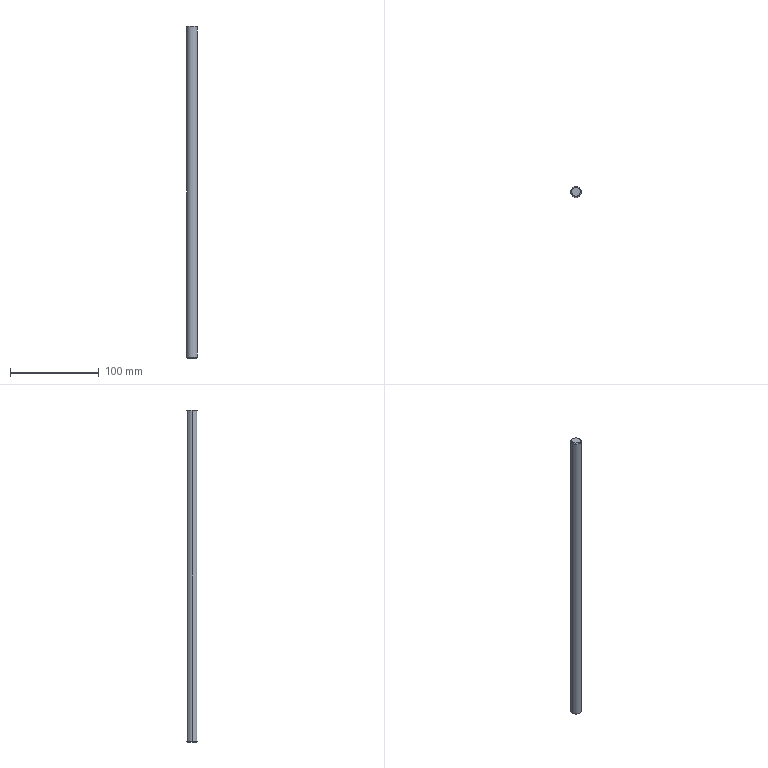Part | SolidWorks | features BaseBody 1 | 1 solid | 20 faces | box 12 x 12 x 374 mm | volume 42082 mm3 | cylinder 8 | plane 8 | cone 4 | commonest cylinder face diameters 3 x6 12 x2
STEP:
#1=CARTESIAN_POINT('',(4.2,0.,-179.));
#2=VERTEX_POINT('',#1);
#3=CARTESIAN_POINT('',(4.2,1.5,-177.5));
#4=VERTEX_POINT('',#3);
#5=CARTESIAN_POINT('',(4.2,0.,-177.5));
#6=DIRECTION('',(1.,0.,0.));
#7=DIRECTION('',(0.,0.,-1.));
#8=AXIS2_PLACEMENT_3D('',#5,#6,#7);
#9=CIRCLE('',#8,1.5);
#10=EDGE_CURVE('',#2,#4,#9,.T.);
#11=ORIENTED_EDGE('',*,*,#10,.F.);
#12=CARTESIAN_POINT('',(6.,0.,-179.));
#13=VERTEX_POINT('',#12);
#14=CARTESIAN_POINT('',(4.2,0.,-179.));
#15=DIRECTION('',(1.,0.,0.));
#16=VECTOR('',#15,1000.);
#17=LINE('',#14,#16);
#18=EDGE_CURVE('',#2,#13,#17,.T.);
#19=ORIENTED_EDGE('',*,*,#18,.T.);
#20=CARTESIAN_POINT('',(5.809,1.5,-177.5));
#21=VERTEX_POINT('',#20);
#22=CARTESIAN_POINT('',(5.809,1.5,-177.5));
#23=CARTESIAN_POINT('',(5.809,1.5,-177.6));
#24=CARTESIAN_POINT('',(5.812,1.49,-177.697));
#25=CARTESIAN_POINT('',(5.822,1.452,-177.89));
#26=CARTESIAN_POINT('',(5.829,1.423,-177.985));
#27=CARTESIAN_POINT('',(5.847,1.347,-178.167));
#28=CARTESIAN_POINT('',(5.857,1.301,-178.253));
#29=CARTESIAN_POINT('',(5.881,1.192,-178.415));
#30=CARTESIAN_POINT('',(5.893,1.129,-178.492));
#31=CARTESIAN_POINT('',(5.93,0.9223,-178.699));
#32=CARTESIAN_POINT('',(5.955,0.7555,-178.81));
#33=CARTESIAN_POINT('',(5.99,0.3946,-178.96));
#34=CARTESIAN_POINT('',(6.,0.1966,-179.));
#35=CARTESIAN_POINT('',(6.,0.,-179.));
#36=B_SPLINE_CURVE_WITH_KNOTS('',3,(#22,#23,#24,#25,#26,#27,#28,#29,#30,#31,#32,#33,#34,#35),.UNSPECIFIED.,.F.,.F.,(4,2,2,2,2,2,4),(0.,0.0002944,0.0005887,0.0008831,0.001177,0.001766,0.002355),.UNSPECIFIED.);
#37=EDGE_CURVE('',#21,#13,#36,.T.);
#38=ORIENTED_EDGE('',*,*,#37,.F.);
#39=CARTESIAN_POINT('',(4.2,1.5,-177.5));
#40=DIRECTION('',(1.,0.,0.));
#41=VECTOR('',#40,1000.);
#42=LINE('',#39,#41);
#43=EDGE_CURVE('',#4,#21,#42,.T.);
#44=ORIENTED_EDGE('',*,*,#43,.F.);
#45=EDGE_LOOP('',(#11,#19,#38,#44));
#46=FACE_OUTER_BOUND('',#45,.T.);
#47=CARTESIAN_POINT('',(4.2,0.,-177.5));
#48=DIRECTION('',(1.,0.,0.));
#49=DIRECTION('',(0.,0.,-1.));
#50=AXIS2_PLACEMENT_3D('',#47,#48,#49);
#51=CYLINDRICAL_SURFACE('',#50,1.5);
#52=ADVANCED_FACE('',(#46),#51,.F.);
#53=CARTESIAN_POINT('',(4.2,0.,161.));
#54=VERTEX_POINT('',#53);
#55=CARTESIAN_POINT('',(4.2,1.5,162.5));
#56=VERTEX_POINT('',#55);
#57=CARTESIAN_POINT('',(4.2,0.,162.5));
#58=DIRECTION('',(1.,0.,0.));
#59=DIRECTION('',(0.,0.,1.));
#60=AXIS2_PLACEMENT_3D('',#57,#58,#59);
#61=CIRCLE('',#60,1.5);
#62=EDGE_CURVE('',#54,#56,#61,.T.);
#63=ORIENTED_EDGE('',*,*,#62,.F.);
#64=CARTESIAN_POINT('',(6.,0.,161.));
#65=VERTEX_POINT('',#64);
#66=CARTESIAN_POINT('',(4.2,0.,161.));
#67=DIRECTION('',(1.,0.,0.));
#68=VECTOR('',#67,1000.);
#69=LINE('',#66,#68);
#70=EDGE_CURVE('',#54,#65,#69,.T.);
#71=ORIENTED_EDGE('',*,*,#70,.T.);
#72=CARTESIAN_POINT('',(5.809,1.5,162.5));
#73=VERTEX_POINT('',#72);
#74=CARTESIAN_POINT('',(5.809,1.5,162.5));
#75=CARTESIAN_POINT('',(5.809,1.5,162.4));
#76=CARTESIAN_POINT('',(5.812,1.49,162.303));
#77=CARTESIAN_POINT('',(5.822,1.452,162.11));
#78=CARTESIAN_POINT('',(5.829,1.423,162.015));
#79=CARTESIAN_POINT('',(5.847,1.347,161.833));
#80=CARTESIAN_POINT('',(5.857,1.301,161.747));
#81=CARTESIAN_POINT('',(5.881,1.192,161.585));
#82=CARTESIAN_POINT('',(5.893,1.129,161.508));
#83=CARTESIAN_POINT('',(5.93,0.9223,161.301));
#84=CARTESIAN_POINT('',(5.955,0.7555,161.19));
#85=CARTESIAN_POINT('',(5.99,0.3946,161.04));
#86=CARTESIAN_POINT('',(6.,0.1966,161.));
#87=CARTESIAN_POINT('',(6.,0.,161.));
#88=B_SPLINE_CURVE_WITH_KNOTS('',3,(#74,#75,#76,#77,#78,#79,#80,#81,#82,#83,#84,#85,#86,#87),.UNSPECIFIED.,.F.,.F.,(4,2,2,2,2,2,4),(0.,0.0002944,0.0005887,0.0008831,0.001177,0.001766,0.002355),.UNSPECIFIED.);
#89=EDGE_CURVE('',#73,#65,#88,.T.);
#90=ORIENTED_EDGE('',*,*,#89,.F.);
#91=CARTESIAN_POINT('',(4.2,1.5,162.5));
#92=DIRECTION('',(1.,0.,0.));
#93=VECTOR('',#92,1000.);
#94=LINE('',#91,#93);
#95=EDGE_CURVE('',#56,#73,#94,.T.);
#96=ORIENTED_EDGE('',*,*,#95,.F.);
#97=EDGE_LOOP('',(#63,#71,#90,#96));
#98=FACE_OUTER_BOUND('',#97,.T.);
#99=CARTESIAN_POINT('',(4.2,0.,162.5));
#100=DIRECTION('',(1.,0.,0.));
#101=DIRECTION('',(0.,0.,-1.));
#102=AXIS2_PLACEMENT_3D('',#99,#100,#101);
#103=CYLINDRICAL_SURFACE('',#102,1.5);
#104=ADVANCED_FACE('',(#98),#103,.F.);
#105=CARTESIAN_POINT('',(-5.,0.,-187.));
#106=VERTEX_POINT('',#105);
#107=CARTESIAN_POINT('',(5.,0.,-187.));
#108=VERTEX_POINT('',#107);
#109=CARTESIAN_POINT('',(0.,0.,-187.));
#110=DIRECTION('',(0.,0.,-1.));
#111=DIRECTION('',(1.,0.,0.));
#112=AXIS2_PLACEMENT_3D('',#109,#110,#111);
#113=CIRCLE('',#112,5.);
#114=EDGE_CURVE('',#106,#108,#113,.T.);
#115=ORIENTED_EDGE('',*,*,#114,.F.);
#116=CARTESIAN_POINT('',(-6.,0.,-186.));
#117=VERTEX_POINT('',#116);
#118=CARTESIAN_POINT('',(-6.,0.,-186.));
#119=DIRECTION('',(-0.7071,0.,0.7071));
#120=VECTOR('',#119,1000.);
#121=LINE('',#118,#120);
#122=EDGE_CURVE('',#106,#117,#121,.T.);
#123=ORIENTED_EDGE('',*,*,#122,.T.);
#124=CARTESIAN_POINT('',(6.,0.,-186.));
#125=VERTEX_POINT('',#124);
#126=CARTESIAN_POINT('',(0.,0.,-186.));
#127=DIRECTION('',(0.,0.,1.));
#128=DIRECTION('',(1.,0.,0.));
#129=AXIS2_PLACEMENT_3D('',#126,#127,#128);
#130=CIRCLE('',#129,6.);
#131=EDGE_CURVE('',#125,#117,#130,.T.);
#132=ORIENTED_EDGE('',*,*,#131,.F.);
#133=CARTESIAN_POINT('',(6.,0.,-186.));
#134=DIRECTION('',(0.7071,0.,0.7071));
#135=VECTOR('',#134,1000.);
#136=LINE('',#133,#135);
#137=EDGE_CURVE('',#108,#125,#136,.T.);
#138=ORIENTED_EDGE('',*,*,#137,.F.);
#139=EDGE_LOOP('',(#115,#123,#132,#138));
#140=FACE_OUTER_BOUND('',#139,.T.);
#141=CARTESIAN_POINT('',(0.,0.,-186.));
#142=DIRECTION('',(0.,0.,1.));
#143=DIRECTION('',(1.,0.,0.));
#144=AXIS2_PLACEMENT_3D('',#141,#142,#143);
#145=CONICAL_SURFACE('',#144,6.,0.7854);
#146=ADVANCED_FACE('',(#140),#145,.T.);
#147=CARTESIAN_POINT('',(5.,0.,187.));
#148=VERTEX_POINT('',#147);
#149=CARTESIAN_POINT('',(-5.,0.,187.));
#150=VERTEX_POINT('',#149);
#151=CARTESIAN_POINT('',(0.,0.,187.));
#152=DIRECTION('',(0.,0.,1.));
#153=DIRECTION('',(1.,0.,0.));
#154=AXIS2_PLACEMENT_3D('',#151,#152,#153);
#155=CIRCLE('',#154,5.);
#156=EDGE_CURVE('',#148,#150,#155,.T.);
#157=ORIENTED_EDGE('',*,*,#156,.F.);
#158=CARTESIAN_POINT('',(6.,0.,186.));
#159=VERTEX_POINT('',#158);
#160=CARTESIAN_POINT('',(5.,0.,187.));
#161=DIRECTION('',(0.7071,0.,-0.7071));
#162=VECTOR('',#161,1000.);
#163=LINE('',#160,#162);
#164=EDGE_CURVE('',#148,#159,#163,.T.);
#165=ORIENTED_EDGE('',*,*,#164,.T.);
#166=CARTESIAN_POINT('',(-6.,0.,186.));
#167=VERTEX_POINT('',#166);
#168=CARTESIAN_POINT('',(0.,0.,186.));
#169=DIRECTION('',(0.,0.,-1.));
#170=DIRECTION('',(1.,0.,0.));
#171=AXIS2_PLACEMENT_3D('',#168,#169,#170);
#172=CIRCLE('',#171,6.);
#173=EDGE_CURVE('',#167,#159,#172,.T.);
#174=ORIENTED_EDGE('',*,*,#173,.F.);
#175=CARTESIAN_POINT('',(-5.,0.,187.));
#176=DIRECTION('',(-0.7071,0.,-0.7071));
#177=VECTOR('',#176,1000.);
#178=LINE('',#175,#177);
#179=EDGE_CURVE('',#150,#167,#178,.T.);
#180=ORIENTED_EDGE('',*,*,#179,.F.);
#181=EDGE_LOOP('',(#157,#165,#174,#180));
#182=FACE_OUTER_BOUND('',#181,.T.);
#183=CARTESIAN_POINT('',(0.,0.,187.));
#184=DIRECTION('',(0.,0.,-1.));
#185=DIRECTION('',(-1.,0.,0.));
#186=AXIS2_PLACEMENT_3D('',#183,#184,#185);
#187=CONICAL_SURFACE('',#186,5.,0.7854);
#188=ADVANCED_FACE('',(#182),#187,.T.);
#189=ORIENTED_EDGE('',*,*,#173,.T.);
#190=CARTESIAN_POINT('',(6.,0.,179.));
#191=VERTEX_POINT('',#190);
#192=CARTESIAN_POINT('',(6.,0.,187.));
#193=DIRECTION('',(0.,0.,-1.));
#194=VECTOR('',#193,1000.);
#195=LINE('',#192,#194);
#196=EDGE_CURVE('',#159,#191,#195,.T.);
#197=ORIENTED_EDGE('',*,*,#196,.T.);
#198=CARTESIAN_POINT('',(5.809,1.5,177.5));
#199=VERTEX_POINT('',#198);
#200=CARTESIAN_POINT('',(6.,0.,179.));
#201=CARTESIAN_POINT('',(6.,0.1962,179.));
#202=CARTESIAN_POINT('',(5.99,0.3944,178.96));
#203=CARTESIAN_POINT('',(5.964,0.6654,178.848));
#204=CARTESIAN_POINT('',(5.953,0.7532,178.801));
#205=CARTESIAN_POINT('',(5.93,0.916,178.692));
#206=CARTESIAN_POINT('',(5.918,0.9912,178.63));
#207=CARTESIAN_POINT('',(5.893,1.13,178.492));
#208=CARTESIAN_POINT('',(5.881,1.193,178.415));
#209=CARTESIAN_POINT('',(5.858,1.301,178.253));
#210=CARTESIAN_POINT('',(5.847,1.347,178.167));
#211=CARTESIAN_POINT('',(5.82,1.461,177.893));
#212=CARTESIAN_POINT('',(5.809,1.5,177.698));
#213=CARTESIAN_POINT('',(5.809,1.5,177.5));
#214=B_SPLINE_CURVE_WITH_KNOTS('',3,(#200,#201,#202,#203,#204,#205,#206,#207,#208,#209,#210,#211,#212,#213),.UNSPECIFIED.,.F.,.F.,(4,2,2,2,2,2,4),(0.004708,0.005297,0.005591,0.005885,0.00618,0.006474,0.007062),.UNSPECIFIED.);
#215=EDGE_CURVE('',#191,#199,#214,.T.);
#216=ORIENTED_EDGE('',*,*,#215,.T.);
#217=CARTESIAN_POINT('',(5.809,1.5,187.));
#218=DIRECTION('',(0.,0.,-1.));
#219=VECTOR('',#218,1000.);
#220=LINE('',#217,#219);
#221=EDGE_CURVE('',#199,#73,#220,.T.);
#222=ORIENTED_EDGE('',*,*,#221,.T.);
#223=ORIENTED_EDGE('',*,*,#89,.T.);
#224=CARTESIAN_POINT('',(6.,0.,-161.));
#225=VERTEX_POINT('',#224);
#226=CARTESIAN_POINT('',(6.,0.,187.));
#227=DIRECTION('',(0.,0.,-1.));
#228=VECTOR('',#227,1000.);
#229=LINE('',#226,#228);
#230=EDGE_CURVE('',#65,#225,#229,.T.);
#231=ORIENTED_EDGE('',*,*,#230,.T.);
#232=CARTESIAN_POINT('',(5.809,1.5,-162.5));
#233=VERTEX_POINT('',#232);
#234=CARTESIAN_POINT('',(6.,0.,-161.));
#235=CARTESIAN_POINT('',(6.,0.1962,-161.));
#236=CARTESIAN_POINT('',(5.99,0.3944,-161.04));
#237=CARTESIAN_POINT('',(5.964,0.6654,-161.152));
#238=CARTESIAN_POINT('',(5.953,0.7532,-161.199));
#239=CARTESIAN_POINT('',(5.93,0.916,-161.308));
#240=CARTESIAN_POINT('',(5.918,0.9912,-161.37));
#241=CARTESIAN_POINT('',(5.893,1.13,-161.508));
#242=CARTESIAN_POINT('',(5.881,1.193,-161.585));
#243=CARTESIAN_POINT('',(5.858,1.301,-161.747));
#244=CARTESIAN_POINT('',(5.847,1.347,-161.833));
#245=CARTESIAN_POINT('',(5.82,1.461,-162.107));
#246=CARTESIAN_POINT('',(5.809,1.5,-162.302));
#247=CARTESIAN_POINT('',(5.809,1.5,-162.5));
#248=B_SPLINE_CURVE_WITH_KNOTS('',3,(#234,#235,#236,#237,#238,#239,#240,#241,#242,#243,#244,#245,#246,#247),.UNSPECIFIED.,.F.,.F.,(4,2,2,2,2,2,4),(0.004708,0.005297,0.005591,0.005885,0.00618,0.006474,0.007062),.UNSPECIFIED.);
#249=EDGE_CURVE('',#225,#233,#248,.T.);
#250=ORIENTED_EDGE('',*,*,#249,.T.);
#251=CARTESIAN_POINT('',(5.809,1.5,187.));
#252=DIRECTION('',(0.,0.,-1.));
#253=VECTOR('',#252,1000.);
#254=LINE('',#251,#253);
#255=EDGE_CURVE('',#233,#21,#254,.T.);
#256=ORIENTED_EDGE('',*,*,#255,.T.);
#257=ORIENTED_EDGE('',*,*,#37,.T.);
#258=CARTESIAN_POINT('',(6.,0.,187.));
#259=DIRECTION('',(0.,0.,-1.));
#260=VECTOR('',#259,1000.);
#261=LINE('',#258,#260);
#262=EDGE_CURVE('',#13,#125,#261,.T.);
#263=ORIENTED_EDGE('',*,*,#262,.T.);
#264=ORIENTED_EDGE('',*,*,#131,.T.);
#265=CARTESIAN_POINT('',(-6.,0.,187.));
#266=DIRECTION('',(0.,0.,-1.));
#267=VECTOR('',#266,1000.);
#268=LINE('',#265,#267);
#269=EDGE_CURVE('',#167,#117,#268,.T.);
#270=ORIENTED_EDGE('',*,*,#269,.F.);
#271=EDGE_LOOP('',(#189,#197,#216,#222,#223,#231,#250,#256,#257,#263,#264,#270));
#272=FACE_OUTER_BOUND('',#271,.T.);
#273=CARTESIAN_POINT('',(0.,0.,187.));
#274=DIRECTION('',(0.,0.,-1.));
#275=DIRECTION('',(-1.,0.,0.));
#276=AXIS2_PLACEMENT_3D('',#273,#274,#275);
#277=CYLINDRICAL_SURFACE('',#276,6.);
#278=ADVANCED_FACE('',(#272),#277,.T.);
#279=ORIENTED_EDGE('',*,*,#196,.F.);
#280=CARTESIAN_POINT('',(0.,0.,186.));
#281=DIRECTION('',(0.,0.,-1.));
#282=DIRECTION('',(1.,0.,0.));
#283=AXIS2_PLACEMENT_3D('',#280,#281,#282);
#284=CIRCLE('',#283,6.);
#285=EDGE_CURVE('',#159,#167,#284,.T.);
#286=ORIENTED_EDGE('',*,*,#285,.T.);
#287=ORIENTED_EDGE('',*,*,#269,.T.);
#288=CARTESIAN_POINT('',(0.,0.,-186.));
#289=DIRECTION('',(0.,0.,1.));
#290=DIRECTION('',(1.,0.,0.));
#291=AXIS2_PLACEMENT_3D('',#288,#289,#290);
#292=CIRCLE('',#291,6.);
#293=EDGE_CURVE('',#117,#125,#292,.T.);
#294=ORIENTED_EDGE('',*,*,#293,.T.);
#295=ORIENTED_EDGE('',*,*,#262,.F.);
#296=CARTESIAN_POINT('',(5.809,-1.5,-177.5));
#297=VERTEX_POINT('',#296);
#298=CARTESIAN_POINT('',(6.,0.,-179.));
#299=CARTESIAN_POINT('',(6.,-0.0982,-179.));
#300=CARTESIAN_POINT('',(5.998,-0.198,-178.99));
#301=CARTESIAN_POINT('',(5.988,-0.3905,-178.952));
#302=CARTESIAN_POINT('',(5.981,-0.4841,-178.923));
#303=CARTESIAN_POINT('',(5.955,-0.7571,-178.81));
#304=CARTESIAN_POINT('',(5.93,-0.9218,-178.699));
#305=CARTESIAN_POINT('',(5.893,-1.13,-178.491));
#306=CARTESIAN_POINT('',(5.881,-1.192,-178.416));
#307=CARTESIAN_POINT('',(5.858,-1.3,-178.254));
#308=CARTESIAN_POINT('',(5.847,-1.347,-178.166));
#309=CARTESIAN_POINT('',(5.82,-1.46,-177.895));
#310=CARTESIAN_POINT('',(5.809,-1.5,-177.699));
#311=CARTESIAN_POINT('',(5.809,-1.5,-177.5));
#312=B_SPLINE_CURVE_WITH_KNOTS('',3,(#298,#299,#300,#301,#302,#303,#304,#305,#306,#307,#308,#309,#310,#311),.UNSPECIFIED.,.F.,.F.,(4,2,2,2,2,2,4),(0.002355,0.002649,0.002943,0.003531,0.003825,0.004119,0.004707),.UNSPECIFIED.);
#313=EDGE_CURVE('',#13,#297,#312,.T.);
#314=ORIENTED_EDGE('',*,*,#313,.T.);
#315=CARTESIAN_POINT('',(5.809,-1.5,-162.5));
#316=VERTEX_POINT('',#315);
#317=CARTESIAN_POINT('',(5.809,-1.5,187.));
#318=DIRECTION('',(0.,0.,1.));
#319=VECTOR('',#318,1000.);
#320=LINE('',#317,#319);
#321=EDGE_CURVE('',#297,#316,#320,.T.);
#322=ORIENTED_EDGE('',*,*,#321,.T.);
#323=CARTESIAN_POINT('',(5.809,-1.5,-162.5));
#324=CARTESIAN_POINT('',(5.809,-1.5,-162.402));
#325=CARTESIAN_POINT('',(5.812,-1.49,-162.302));
#326=CARTESIAN_POINT('',(5.822,-1.452,-162.109));
#327=CARTESIAN_POINT('',(5.829,-1.423,-162.016));
#328=CARTESIAN_POINT('',(5.856,-1.31,-161.743));
#329=CARTESIAN_POINT('',(5.881,-1.199,-161.578));
#330=CARTESIAN_POINT('',(5.918,-0.9907,-161.369));
#331=CARTESIAN_POINT('',(5.93,-0.9154,-161.308));
#332=CARTESIAN_POINT('',(5.953,-0.7533,-161.199));
#333=CARTESIAN_POINT('',(5.964,-0.6654,-161.152));
#334=CARTESIAN_POINT('',(5.981,-0.4843,-161.077));
#335=CARTESIAN_POINT('',(5.988,-0.3908,-161.048));
#336=CARTESIAN_POINT('',(5.998,-0.1977,-161.01));
#337=CARTESIAN_POINT('',(6.,-0.0981,-161.));
#338=CARTESIAN_POINT('',(6.,0.,-161.));
#339=B_SPLINE_CURVE_WITH_KNOTS('',3,(#323,#324,#325,#326,#327,#328,#329,#330,#331,#332,#333,#334,#335,#336,#337,#338),.UNSPECIFIED.,.F.,.F.,(4,2,2,2,2,2,2,4),(0.002355,0.002649,0.002943,0.003532,0.003826,0.00412,0.004414,0.004708),.UNSPECIFIED.);
#340=EDGE_CURVE('',#316,#225,#339,.T.);
#341=ORIENTED_EDGE('',*,*,#340,.T.);
#342=ORIENTED_EDGE('',*,*,#230,.F.);
#343=CARTESIAN_POINT('',(5.809,-1.5,162.5));
#344=VERTEX_POINT('',#343);
#345=CARTESIAN_POINT('',(6.,0.,161.));
#346=CARTESIAN_POINT('',(6.,-0.0982,161.));
#347=CARTESIAN_POINT('',(5.998,-0.198,161.01));
#348=CARTESIAN_POINT('',(5.988,-0.3905,161.048));
#349=CARTESIAN_POINT('',(5.981,-0.4841,161.077));
#350=CARTESIAN_POINT('',(5.955,-0.7571,161.19));
#351=CARTESIAN_POINT('',(5.93,-0.9218,161.301));
#352=CARTESIAN_POINT('',(5.893,-1.13,161.509));
#353=CARTESIAN_POINT('',(5.881,-1.192,161.584));
#354=CARTESIAN_POINT('',(5.858,-1.3,161.746));
#355=CARTESIAN_POINT('',(5.847,-1.347,161.834));
#356=CARTESIAN_POINT('',(5.82,-1.46,162.105));
#357=CARTESIAN_POINT('',(5.809,-1.5,162.301));
#358=CARTESIAN_POINT('',(5.809,-1.5,162.5));
#359=B_SPLINE_CURVE_WITH_KNOTS('',3,(#345,#346,#347,#348,#349,#350,#351,#352,#353,#354,#355,#356,#357,#358),.UNSPECIFIED.,.F.,.F.,(4,2,2,2,2,2,4),(0.002355,0.002649,0.002943,0.003531,0.003825,0.004119,0.004707),.UNSPECIFIED.);
#360=EDGE_CURVE('',#65,#344,#359,.T.);
#361=ORIENTED_EDGE('',*,*,#360,.T.);
#362=CARTESIAN_POINT('',(5.809,-1.5,177.5));
#363=VERTEX_POINT('',#362);
#364=CARTESIAN_POINT('',(5.809,-1.5,187.));
#365=DIRECTION('',(0.,0.,1.));
#366=VECTOR('',#365,1000.);
#367=LINE('',#364,#366);
#368=EDGE_CURVE('',#344,#363,#367,.T.);
#369=ORIENTED_EDGE('',*,*,#368,.T.);
#370=CARTESIAN_POINT('',(5.809,-1.5,177.5));
#371=CARTESIAN_POINT('',(5.809,-1.5,177.598));
#372=CARTESIAN_POINT('',(5.812,-1.49,177.698));
#373=CARTESIAN_POINT('',(5.822,-1.452,177.891));
#374=CARTESIAN_POINT('',(5.829,-1.423,177.984));
#375=CARTESIAN_POINT('',(5.856,-1.31,178.257));
#376=CARTESIAN_POINT('',(5.881,-1.199,178.422));
#377=CARTESIAN_POINT('',(5.918,-0.9907,178.631));
#378=CARTESIAN_POINT('',(5.93,-0.9154,178.692));
#379=CARTESIAN_POINT('',(5.953,-0.7533,178.801));
#380=CARTESIAN_POINT('',(5.964,-0.6654,178.848));
#381=CARTESIAN_POINT('',(5.981,-0.4843,178.923));
#382=CARTESIAN_POINT('',(5.988,-0.3908,178.952));
#383=CARTESIAN_POINT('',(5.998,-0.1977,178.99));
#384=CARTESIAN_POINT('',(6.,-0.0981,179.));
#385=CARTESIAN_POINT('',(6.,0.,179.));
#386=B_SPLINE_CURVE_WITH_KNOTS('',3,(#370,#371,#372,#373,#374,#375,#376,#377,#378,#379,#380,#381,#382,#383,#384,#385),.UNSPECIFIED.,.F.,.F.,(4,2,2,2,2,2,2,4),(0.002355,0.002649,0.002943,0.003532,0.003826,0.00412,0.004414,0.004708),.UNSPECIFIED.);
#387=EDGE_CURVE('',#363,#191,#386,.T.);
#388=ORIENTED_EDGE('',*,*,#387,.T.);
#389=EDGE_LOOP('',(#279,#286,#287,#294,#295,#314,#322,#341,#342,#361,#369,#388));
#390=FACE_OUTER_BOUND('',#389,.T.);
#391=CARTESIAN_POINT('',(0.,0.,187.));
#392=DIRECTION('',(0.,0.,-1.));
#393=DIRECTION('',(-1.,0.,0.));
#394=AXIS2_PLACEMENT_3D('',#391,#392,#393);
#395=CYLINDRICAL_SURFACE('',#394,6.);
#396=ADVANCED_FACE('',(#390),#395,.T.);
#397=CARTESIAN_POINT('',(0.,0.,187.));
#398=DIRECTION('',(0.,0.,1.));
#399=DIRECTION('',(1.,0.,0.));
#400=AXIS2_PLACEMENT_3D('',#397,#398,#399);
#401=CIRCLE('',#400,5.);
#402=EDGE_CURVE('',#150,#148,#401,.T.);
#403=ORIENTED_EDGE('',*,*,#402,.T.);
#404=ORIENTED_EDGE('',*,*,#156,.T.);
#405=EDGE_LOOP('',(#403,#404));
#406=FACE_OUTER_BOUND('',#405,.T.);
#407=CARTESIAN_POINT('',(0.,0.,187.));
#408=DIRECTION('',(0.,0.,1.));
#409=DIRECTION('',(1.,0.,0.));
#410=AXIS2_PLACEMENT_3D('',#407,#408,#409);
#411=PLANE('',#410);
#412=ADVANCED_FACE('',(#406),#411,.T.);
#413=CARTESIAN_POINT('',(0.,0.,-187.));
#414=DIRECTION('',(0.,0.,-1.));
#415=DIRECTION('',(1.,0.,0.));
#416=AXIS2_PLACEMENT_3D('',#413,#414,#415);
#417=CIRCLE('',#416,5.);
#418=EDGE_CURVE('',#108,#106,#417,.T.);
#419=ORIENTED_EDGE('',*,*,#418,.T.);
#420=ORIENTED_EDGE('',*,*,#114,.T.);
#421=EDGE_LOOP('',(#419,#420));
#422=FACE_OUTER_BOUND('',#421,.T.);
#423=CARTESIAN_POINT('',(0.,0.,-187.));
#424=DIRECTION('',(0.,0.,1.));
#425=DIRECTION('',(1.,0.,0.));
#426=AXIS2_PLACEMENT_3D('',#423,#424,#425);
#427=PLANE('',#426);
#428=ADVANCED_FACE('',(#422),#427,.F.);
#429=ORIENTED_EDGE('',*,*,#164,.F.);
#430=ORIENTED_EDGE('',*,*,#402,.F.);
#431=ORIENTED_EDGE('',*,*,#179,.T.);
#432=ORIENTED_EDGE('',*,*,#285,.F.);
#433=EDGE_LOOP('',(#429,#430,#431,#432));
#434=FACE_OUTER_BOUND('',#433,.T.);
#435=CARTESIAN_POINT('',(0.,0.,187.));
#436=DIRECTION('',(0.,0.,-1.));
#437=DIRECTION('',(-1.,0.,0.));
#438=AXIS2_PLACEMENT_3D('',#435,#436,#437);
#439=CONICAL_SURFACE('',#438,5.,0.7854);
#440=ADVANCED_FACE('',(#434),#439,.T.);
#441=ORIENTED_EDGE('',*,*,#122,.F.);
#442=ORIENTED_EDGE('',*,*,#418,.F.);
#443=ORIENTED_EDGE('',*,*,#137,.T.);
#444=ORIENTED_EDGE('',*,*,#293,.F.);
#445=EDGE_LOOP('',(#441,#442,#443,#444));
#446=FACE_OUTER_BOUND('',#445,.T.);
#447=CARTESIAN_POINT('',(0.,0.,-186.));
#448=DIRECTION('',(0.,0.,1.));
#449=DIRECTION('',(1.,0.,0.));
#450=AXIS2_PLACEMENT_3D('',#447,#448,#449);
#451=CONICAL_SURFACE('',#450,6.,0.7854);
#452=ADVANCED_FACE('',(#446),#451,.T.);
#453=CARTESIAN_POINT('',(4.2,-1.5,177.5));
#454=VERTEX_POINT('',#453);
#455=CARTESIAN_POINT('',(4.2,-1.5,177.5));
#456=DIRECTION('',(1.,0.,0.));
#457=VECTOR('',#456,1000.);
#458=LINE('',#455,#457);
#459=EDGE_CURVE('',#454,#363,#458,.T.);
#460=ORIENTED_EDGE('',*,*,#459,.F.);
#461=CARTESIAN_POINT('',(4.2,1.5,177.5));
#462=VERTEX_POINT('',#461);
#463=CARTESIAN_POINT('',(4.2,0.,177.5));
#464=DIRECTION('',(1.,0.,0.));
#465=DIRECTION('',(0.,0.,1.));
#466=AXIS2_PLACEMENT_3D('',#463,#464,#465);
#467=CIRCLE('',#466,1.5);
#468=EDGE_CURVE('',#462,#454,#467,.T.);
#469=ORIENTED_EDGE('',*,*,#468,.F.);
#470=CARTESIAN_POINT('',(4.2,1.5,177.5));
#471=DIRECTION('',(1.,0.,0.));
#472=VECTOR('',#471,1000.);
#473=LINE('',#470,#472);
#474=EDGE_CURVE('',#462,#199,#473,.T.);
#475=ORIENTED_EDGE('',*,*,#474,.T.);
#476=ORIENTED_EDGE('',*,*,#215,.F.);
#477=ORIENTED_EDGE('',*,*,#387,.F.);
#478=EDGE_LOOP('',(#460,#469,#475,#476,#477));
#479=FACE_OUTER_BOUND('',#478,.T.);
#480=CARTESIAN_POINT('',(4.2,0.,177.5));
#481=DIRECTION('',(1.,0.,0.));
#482=DIRECTION('',(0.,0.,-1.));
#483=AXIS2_PLACEMENT_3D('',#480,#481,#482);
#484=CYLINDRICAL_SURFACE('',#483,1.5);
#485=ADVANCED_FACE('',(#479),#484,.F.);
#486=ORIENTED_EDGE('',*,*,#474,.F.);
#487=CARTESIAN_POINT('',(4.2,1.5,177.5));
#488=DIRECTION('',(0.,0.,1.));
#489=VECTOR('',#488,1000.);
#490=LINE('',#487,#489);
#491=EDGE_CURVE('',#56,#462,#490,.T.);
#492=ORIENTED_EDGE('',*,*,#491,.F.);
#493=ORIENTED_EDGE('',*,*,#95,.T.);
#494=ORIENTED_EDGE('',*,*,#221,.F.);
#495=EDGE_LOOP('',(#486,#492,#493,#494));
#496=FACE_OUTER_BOUND('',#495,.T.);
#497=CARTESIAN_POINT('',(4.2,1.5,177.5));
#498=DIRECTION('',(0.,1.,0.));
#499=DIRECTION('',(0.,0.,1.));
#500=AXIS2_PLACEMENT_3D('',#497,#498,#499);
#501=PLANE('',#500);
#502=ADVANCED_FACE('',(#496),#501,.F.);
#503=ORIENTED_EDGE('',*,*,#70,.F.);
#504=CARTESIAN_POINT('',(4.2,-1.5,162.5));
#505=VERTEX_POINT('',#504);
#506=CARTESIAN_POINT('',(4.2,0.,162.5));
#507=DIRECTION('',(1.,0.,0.));
#508=DIRECTION('',(0.,0.,1.));
#509=AXIS2_PLACEMENT_3D('',#506,#507,#508);
#510=CIRCLE('',#509,1.5);
#511=EDGE_CURVE('',#505,#54,#510,.T.);
#512=ORIENTED_EDGE('',*,*,#511,.F.);
#513=CARTESIAN_POINT('',(4.2,-1.5,162.5));
#514=DIRECTION('',(1.,0.,0.));
#515=VECTOR('',#514,1000.);
#516=LINE('',#513,#515);
#517=EDGE_CURVE('',#505,#344,#516,.T.);
#518=ORIENTED_EDGE('',*,*,#517,.T.);
#519=ORIENTED_EDGE('',*,*,#360,.F.);
#520=EDGE_LOOP('',(#503,#512,#518,#519));
#521=FACE_OUTER_BOUND('',#520,.T.);
#522=CARTESIAN_POINT('',(4.2,0.,162.5));
#523=DIRECTION('',(1.,0.,0.));
#524=DIRECTION('',(0.,0.,-1.));
#525=AXIS2_PLACEMENT_3D('',#522,#523,#524);
#526=CYLINDRICAL_SURFACE('',#525,1.5);
#527=ADVANCED_FACE('',(#521),#526,.F.);
#528=ORIENTED_EDGE('',*,*,#517,.F.);
#529=CARTESIAN_POINT('',(4.2,-1.5,177.5));
#530=DIRECTION('',(0.,0.,-1.));
#531=VECTOR('',#530,1000.);
#532=LINE('',#529,#531);
#533=EDGE_CURVE('',#454,#505,#532,.T.);
#534=ORIENTED_EDGE('',*,*,#533,.F.);
#535=ORIENTED_EDGE('',*,*,#459,.T.);
#536=ORIENTED_EDGE('',*,*,#368,.F.);
#537=EDGE_LOOP('',(#528,#534,#535,#536));
#538=FACE_OUTER_BOUND('',#537,.T.);
#539=CARTESIAN_POINT('',(4.2,-1.5,177.5));
#540=DIRECTION('',(0.,-1.,0.));
#541=DIRECTION('',(0.,0.,-1.));
#542=AXIS2_PLACEMENT_3D('',#539,#540,#541);
#543=PLANE('',#542);
#544=ADVANCED_FACE('',(#538),#543,.F.);
#545=ORIENTED_EDGE('',*,*,#468,.T.);
#546=ORIENTED_EDGE('',*,*,#533,.T.);
#547=ORIENTED_EDGE('',*,*,#511,.T.);
#548=ORIENTED_EDGE('',*,*,#62,.T.);
#549=ORIENTED_EDGE('',*,*,#491,.T.);
#550=EDGE_LOOP('',(#545,#546,#547,#548,#549));
#551=FACE_OUTER_BOUND('',#550,.T.);
#552=CARTESIAN_POINT('',(4.2,0.,177.5));
#553=DIRECTION('',(-1.,0.,0.));
#554=DIRECTION('',(0.,0.,1.));
#555=AXIS2_PLACEMENT_3D('',#552,#553,#554);
#556=PLANE('',#555);
#557=ADVANCED_FACE('',(#551),#556,.F.);
#558=ORIENTED_EDGE('',*,*,#18,.F.);
#559=CARTESIAN_POINT('',(4.2,-1.5,-177.5));
#560=VERTEX_POINT('',#559);
#561=CARTESIAN_POINT('',(4.2,0.,-177.5));
#562=DIRECTION('',(1.,0.,0.));
#563=DIRECTION('',(0.,0.,-1.));
#564=AXIS2_PLACEMENT_3D('',#561,#562,#563);
#565=CIRCLE('',#564,1.5);
#566=EDGE_CURVE('',#560,#2,#565,.T.);
#567=ORIENTED_EDGE('',*,*,#566,.F.);
#568=CARTESIAN_POINT('',(4.2,-1.5,-177.5));
#569=DIRECTION('',(1.,0.,0.));
#570=VECTOR('',#569,1000.);
#571=LINE('',#568,#570);
#572=EDGE_CURVE('',#560,#297,#571,.T.);
#573=ORIENTED_EDGE('',*,*,#572,.T.);
#574=ORIENTED_EDGE('',*,*,#313,.F.);
#575=EDGE_LOOP('',(#558,#567,#573,#574));
#576=FACE_OUTER_BOUND('',#575,.T.);
#577=CARTESIAN_POINT('',(4.2,0.,-177.5));
#578=DIRECTION('',(1.,0.,0.));
#579=DIRECTION('',(0.,0.,-1.));
#580=AXIS2_PLACEMENT_3D('',#577,#578,#579);
#581=CYLINDRICAL_SURFACE('',#580,1.5);
#582=ADVANCED_FACE('',(#576),#581,.F.);
#583=ORIENTED_EDGE('',*,*,#572,.F.);
#584=CARTESIAN_POINT('',(4.2,-1.5,-162.5));
#585=VERTEX_POINT('',#584);
#586=CARTESIAN_POINT('',(4.2,-1.5,-177.5));
#587=DIRECTION('',(0.,0.,-1.));
#588=VECTOR('',#587,1000.);
#589=LINE('',#586,#588);
#590=EDGE_CURVE('',#585,#560,#589,.T.);
#591=ORIENTED_EDGE('',*,*,#590,.F.);
#592=CARTESIAN_POINT('',(4.2,-1.5,-162.5));
#593=DIRECTION('',(1.,0.,0.));
#594=VECTOR('',#593,1000.);
#595=LINE('',#592,#594);
#596=EDGE_CURVE('',#585,#316,#595,.T.);
#597=ORIENTED_EDGE('',*,*,#596,.T.);
#598=ORIENTED_EDGE('',*,*,#321,.F.);
#599=EDGE_LOOP('',(#583,#591,#597,#598));
#600=FACE_OUTER_BOUND('',#599,.T.);
#601=CARTESIAN_POINT('',(4.2,-1.5,-177.5));
#602=DIRECTION('',(0.,-1.,0.));
#603=DIRECTION('',(0.,0.,-1.));
#604=AXIS2_PLACEMENT_3D('',#601,#602,#603);
#605=PLANE('',#604);
#606=ADVANCED_FACE('',(#600),#605,.F.);
#607=ORIENTED_EDGE('',*,*,#596,.F.);
#608=CARTESIAN_POINT('',(4.2,1.5,-162.5));
#609=VERTEX_POINT('',#608);
#610=CARTESIAN_POINT('',(4.2,0.,-162.5));
#611=DIRECTION('',(1.,0.,0.));
#612=DIRECTION('',(0.,0.,-1.));
#613=AXIS2_PLACEMENT_3D('',#610,#611,#612);
#614=CIRCLE('',#613,1.5);
#615=EDGE_CURVE('',#609,#585,#614,.T.);
#616=ORIENTED_EDGE('',*,*,#615,.F.);
#617=CARTESIAN_POINT('',(4.2,1.5,-162.5));
#618=DIRECTION('',(1.,0.,0.));
#619=VECTOR('',#618,1000.);
#620=LINE('',#617,#619);
#621=EDGE_CURVE('',#609,#233,#620,.T.);
#622=ORIENTED_EDGE('',*,*,#621,.T.);
#623=ORIENTED_EDGE('',*,*,#249,.F.);
#624=ORIENTED_EDGE('',*,*,#340,.F.);
#625=EDGE_LOOP('',(#607,#616,#622,#623,#624));
#626=FACE_OUTER_BOUND('',#625,.T.);
#627=CARTESIAN_POINT('',(4.2,0.,-162.5));
#628=DIRECTION('',(1.,0.,0.));
#629=DIRECTION('',(0.,0.,-1.));
#630=AXIS2_PLACEMENT_3D('',#627,#628,#629);
#631=CYLINDRICAL_SURFACE('',#630,1.5);
#632=ADVANCED_FACE('',(#626),#631,.F.);
#633=ORIENTED_EDGE('',*,*,#621,.F.);
#634=CARTESIAN_POINT('',(4.2,1.5,-177.5));
#635=DIRECTION('',(0.,0.,1.));
#636=VECTOR('',#635,1000.);
#637=LINE('',#634,#636);
#638=EDGE_CURVE('',#4,#609,#637,.T.);
#639=ORIENTED_EDGE('',*,*,#638,.F.);
#640=ORIENTED_EDGE('',*,*,#43,.T.);
#641=ORIENTED_EDGE('',*,*,#255,.F.);
#642=EDGE_LOOP('',(#633,#639,#640,#641));
#643=FACE_OUTER_BOUND('',#642,.T.);
#644=CARTESIAN_POINT('',(4.2,1.5,-177.5));
#645=DIRECTION('',(0.,1.,0.));
#646=DIRECTION('',(0.,0.,1.));
#647=AXIS2_PLACEMENT_3D('',#644,#645,#646);
#648=PLANE('',#647);
#649=ADVANCED_FACE('',(#643),#648,.F.);
#650=ORIENTED_EDGE('',*,*,#566,.T.);
#651=ORIENTED_EDGE('',*,*,#10,.T.);
#652=ORIENTED_EDGE('',*,*,#638,.T.);
#653=ORIENTED_EDGE('',*,*,#615,.T.);
#654=ORIENTED_EDGE('',*,*,#590,.T.);
#655=EDGE_LOOP('',(#650,#651,#652,#653,#654));
#656=FACE_OUTER_BOUND('',#655,.T.);
#657=CARTESIAN_POINT('',(4.2,0.,-177.5));
#658=DIRECTION('',(1.,0.,0.));
#659=DIRECTION('',(0.,0.,-1.));
#660=AXIS2_PLACEMENT_3D('',#657,#658,#659);
#661=PLANE('',#660);
#662=ADVANCED_FACE('',(#656),#661,.T.);
#663=CLOSED_SHELL('',(#52,#104,#146,#188,#278,#396,#412,#428,#440,#452,#485,#502,#527,#544,#557,#582,#606,#632,#649,#662));
#664=MANIFOLD_SOLID_BREP('',#663);
#665=CARTESIAN_POINT('',(0.,0.,0.));
#666=DIRECTION('',(0.,0.,1.));
#667=DIRECTION('',(1.,0.,0.));
#668=AXIS2_PLACEMENT_3D('',#665,#666,#667);
#669=(LENGTH_UNIT()NAMED_UNIT(*)SI_UNIT(.MILLI.,.METRE.));
#670=UNCERTAINTY_MEASURE_WITH_UNIT(LENGTH_MEASURE(0.00001),#669,'','');
#671=(NAMED_UNIT(*)PLANE_ANGLE_UNIT()SI_UNIT($,.RADIAN.));
#672=(NAMED_UNIT(*)SI_UNIT($,.STERADIAN.)SOLID_ANGLE_UNIT());
#673=(GEOMETRIC_REPRESENTATION_CONTEXT(3)GLOBAL_UNCERTAINTY_ASSIGNED_CONTEXT((#670))GLOBAL_UNIT_ASSIGNED_CONTEXT((#669,#671,#672))REPRESENTATION_CONTEXT('',''));
#674=ADVANCED_BREP_SHAPE_REPRESENTATION('',(#664,#668),#673);